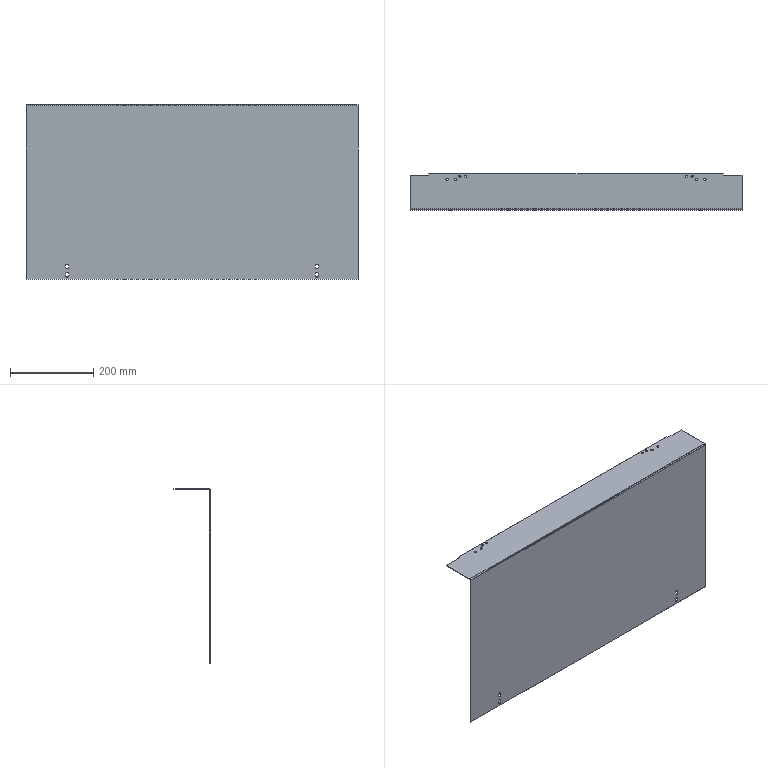Part | STEP file | Small busbar cover | 1 solid | 54 faces | box 798 x 87 x 420 mm | volume 602724 mm3 | cylinder 30 | plane 24 | commonest cylinder face diameters 5.3 x16 7 x12 3 x1 6 x1